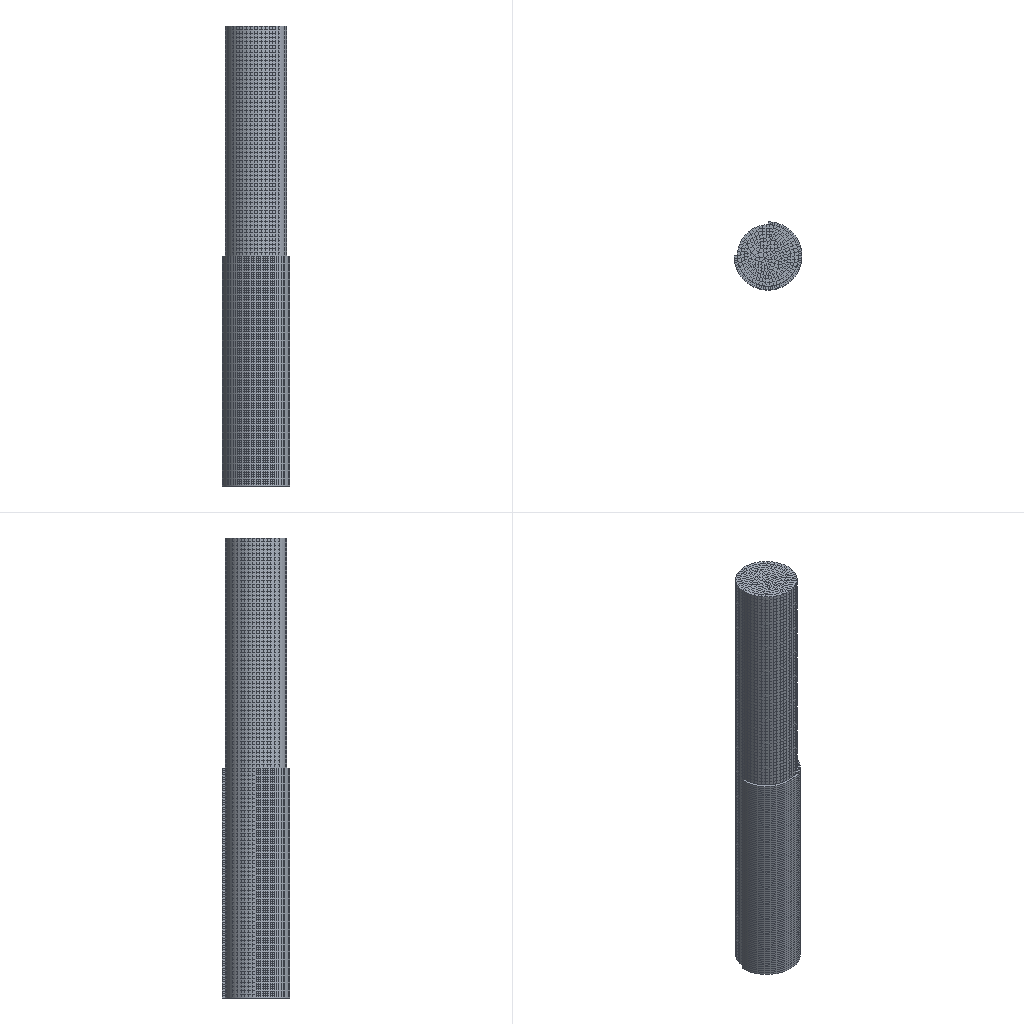Simulation study | abaqus
Set-up summary:
category,name,step,type,value,unit,region
solver,abaqus,,Abaqus/CAE 2024
units,mm-N-s-tonne (MPa),,inferred,E=2000 density=9.1e-10
analysis,Step-1,,static,nlgeom=True; time_period=1
mesh,nodes,,,50077
mesh,elements,,,39720
element_type,C3D8R,,,39720
material,ice,,E,2000
material,ice,,nu,0.3
material,ice,,density,9.1e-10
material,iron,,E,200000
material,iron,,nu,0.3
material,iron,,density,7.85e-09
section,ice,,solid section,,,_PickedSet2
section,iron,,solid section,,,_PickedSet2
bc,BC-1,Step-1,encastre,[dofs=ENCASTRE],,_PickedSet8
bc,BC-3,Step-1,fixed,"[dofs=rx,ry,rz,x,y n=5]",,_PickedSet13
bc,BC-3,Step-1,displacement,2 [dofs=z],,_PickedSet13
contact,Int-1,initial,contact pair,interaction=IntProp-1,,ice-1.Surf-ice / iron-1.Surf-iron
constraint,coupling,,,1
Abaqus input file, long lists of numbers shortened:
*Heading
** Job name: deck Model name: Model-1-Copy
** Generated by: Abaqus/CAE 2024
*Preprint, echo=NO, model=NO, history=NO, contact=NO
**
** PARTS
**
*Part, name=ice
*Node
      1,       -4.421,           0.,          30.
      2,          -4.,           0.,          30.
** (13532 more lines like these left out)
*Element, type=C3D8R
   1,     3,     4,     2,     1,   205,   206,   204,   203
   2,     5,     6,     4,     3,   207,   208,   206,   205
** (6598 more lines like these left out)
*Nset, nset=_PickedSet2, internal, generate
     1,  13534,      1
*Elset, elset=_PickedSet2, internal, generate
    1,  6600,     1
*Elset, elset=_Surf-ice_S4, internal, generate
    1,  6600,     1
*Surface, type=ELEMENT, name=Surf-ice
_Surf-ice_S4, S4
** Section: ice
*Solid Section, elset=_PickedSet2, material=ice
,
*End Part
**
*Part, name=iron
*Node
      1,   3.505,   1.927,           0.
      2,   2.143,   3.377,           0.
** (36540 more lines like these left out)
*Element, type=C3D8R
    1,   384,   346,   345,   383,    82,    44,    43,    81
    2,   379,   341,   340,   411,    77,    39,    38,   109
** (33118 more lines like these left out)
*Nset, nset=_PickedSet2, internal, generate
     1,  36542,      1
*Elset, elset=_PickedSet2, internal, generate
     1,  33120,      1
*Elset, elset=_Surf-iron_S4, internal
     1,     2,     4,    10,    11,    12,    27,    33,    34,    42,    43,    44,    46,   106,   252,   277
   278,   280,   286,   287,   288,   303,   309,   310,   318,   319,   320,   322,   382,   528,   553,   554
** (111 more lines like these left out)
*Elset, elset=_Surf-iron_S6, internal
     5,     6,     8,    13,    14,    24,    25,    28,    29,    30,    31,    32,    35,    36,    37,    38
    40,    45,    47,    52,    65,    71,    82,   251,   281,   282,   284,   289,   290,   300,   301,   304
** (178 more lines like these left out)
*Elset, elset=_Surf-iron_S3, internal
     9,    18,    19,    20,    21,    50,    61,   250,   285,   294,   295,   296,   297,   326,   337,   526
   561,   570,   571,   572,   573,   602,   613,   802,   837,   846,   847,   848,   849,   878,   889,  1078
** (58 more lines like these left out)
*Elset, elset=_Surf-iron_S5, internal
    16,    49,    57,   292,   325,   333,   568,   601,   609,   844,   877,   885,  1120,  1153,  1161,  1396
  1429,  1437,  1672,  1705,  1713,  1948,  1981,  1989,  2224,  2257,  2265,  2500,  2533,  2541,  2776,  2809
** (21 more lines like these left out)
*Surface, type=ELEMENT, name=Surf-iron
_Surf-iron_S4, S4
_Surf-iron_S6, S6
_Surf-iron_S3, S3
_Surf-iron_S5, S5
** Section: iron
*Solid Section, elset=_PickedSet2, material=iron
,
*End Part
**
**
** ASSEMBLY
**
*Assembly, name=Assembly
**
*Instance, name=ice-1, part=ice
*End Instance
**
*Instance, name=iron-1, part=iron
*End Instance
**
*Node
      1,        4.421,           0.,           0.
*Nset, nset=_PickedSet8, internal, instance=iron-1
     1,     2,     3,     4,     5,     6,     7,     8,     9,    10,    11,    12,    13,    14,    15,    16
    17,    18,    19,    20,    21,    22,    23,    24,    25,    26,    27,    28,    29,    30,    31,    32
** (408 more lines like these left out)
*Elset, elset=_PickedSet8, internal, instance=iron-1
     1,     2,     3,     4,     5,     6,     7,     8,     9,    10,    11,    12,    13,    14,    15,    16
    17,    18,    19,    20,    21,    22,    23,    24,    25,    26,    27,    28,    29,    30,    31,    32
** (402 more lines like these left out)
*Nset, nset=_PickedSet11, internal
 1,
*Nset, nset=_PickedSet12, internal
 1,
*Nset, nset=_PickedSet13, internal
 1,
*Elset, elset=__PickedSurf6_S3, internal, instance=ice-1, generate
  100,  6600,   100
*Surface, type=ELEMENT, name=_PickedSurf6, internal
__PickedSurf6_S3, S3
** Constraint: Constraint-1
*Coupling, constraint name=Constraint-1, ref node=_PickedSet11, surface=_PickedSurf6
*Kinematic
*End Assembly
*Amplitude, name=Amp-1
             0.,              1.,              1.,              1.
**
** MATERIALS
**
*Material, name=ice
*Density
 9.1e-10,
*Elastic
2000., 0.3
*Material, name=iron
*Density
 7.85e-09,
*Elastic
200000., 0.3
**
** INTERACTION PROPERTIES
**
*Surface Interaction, name=IntProp-1
1.,
*Cohesive Behavior
90.,90.,90.
*Damage Initiation, criterion=QUADS
 0.05, 0.05, 0.05
*Damage Evolution, type=DISPLACEMENT
 0.1,
*Damage Stabilization
0.05
**
** INTERACTIONS
**
** Interaction: Int-1
*Contact Pair, interaction=IntProp-1, small sliding
ice-1.Surf-ice, iron-1.Surf-iron
** ----------------------------------------------------------------
**
** STEP: Step-1
**
*Step, name=Step-1, nlgeom=YES, inc=10000
*Static
0.01, 1., 1e-10, 0.02
**
** BOUNDARY CONDITIONS
**
** Name: BC-1 Type: Symmetry/Antisymmetry/Encastre
*Boundary
_PickedSet8, ENCASTRE
** Name: BC-3 Type: Displacement/Rotation
*Boundary
_PickedSet13, 1, 1
_PickedSet13, 2, 2
_PickedSet13, 3, 3, 2.
_PickedSet13, 4, 4
_PickedSet13, 5, 5
_PickedSet13, 6, 6
**
** OUTPUT REQUESTS
**
*Restart, write, frequency=0
**
** FIELD OUTPUT: F-Output-1
**
*Output, field
*Node Output
CF, RF, U
*Element Output, directions=YES
DMICRT, LE, PE, PEEQ, PEMAG, S, SDEG
*Contact Output
CDISP, CSQUADSCRT, CSTRESS
**
** HISTORY OUTPUT: H-Output-1
**
*Output, history, variable=PRESELECT
*End Step
Results summary:
result,odb.job_status,,,JOB_STATUS_COMPLETED_SUCCESSFULLY,"consistent, unstated (Abaqus has no unit system)"
result,steps[0].procedure,Step-1,,*STATIC,"consistent, unstated (Abaqus has no unit system)"
result,steps[0].time_period,Step-1,,1,"consistent, unstated (Abaqus has no unit system)"
result,steps[0].n_frames,Step-1,,59,"consistent, unstated (Abaqus has no unit system)"
result,steps[0].last_frame.id,Step-1,,58,"consistent, unstated (Abaqus has no unit system)"
result,steps[0].last_frame.value,Step-1,,1,"consistent, unstated (Abaqus has no unit system)"
result,steps[0].last_frame.description,Step-1,,Increment     58: Step Time =    1.000,"consistent, unstated (Abaqus has no unit system)"
result,steps[0].completed,Step-1,,True,"consistent, unstated (Abaqus has no unit system)"
result,steps[0].max_U_magnitude,Step-1,,2,"consistent, unstated (Abaqus has no unit system)"
result,steps[0].max_S_mises,Step-1,,0.003946,"consistent, unstated (Abaqus has no unit system)"
result,steps[0].RF_sum[1],Step-1,,-9.25183e-10,"consistent, unstated (Abaqus has no unit system)"
result,steps[0].RF_sum[2],Step-1,,-1.9794e-16,"consistent, unstated (Abaqus has no unit system)"
result,steps[0].RF_sum[3],Step-1,,-1.2017e-16,"consistent, unstated (Abaqus has no unit system)"